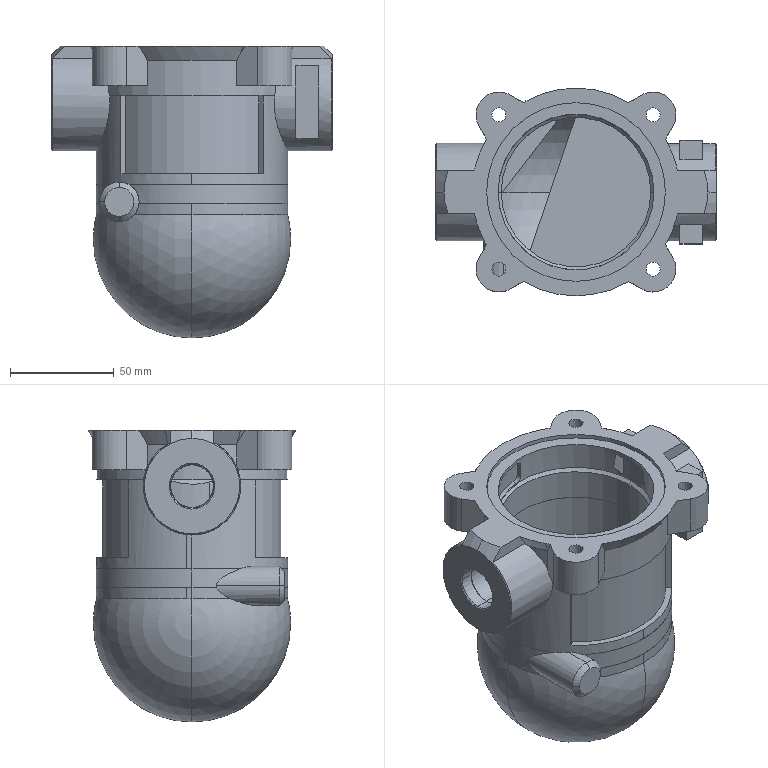Part | SolidWorks | features ICE 9, Fillet 7, HoleWzd 2, Revolution 2, BaseBody 1, Chamfer 1, MirrorPattern 1, RevCut 1 | 1 solid | 219 faces | box 135 x 100 x 140.5 mm | volume 345567 mm3 | cylinder 82 | plane 78 | cone 38 | spline 8 | torus 7 | sphere 6 | commonest cylinder face diameters 92 x19 92.2 x9 6 x8 6.8 x8 20.95 x8 19 x4